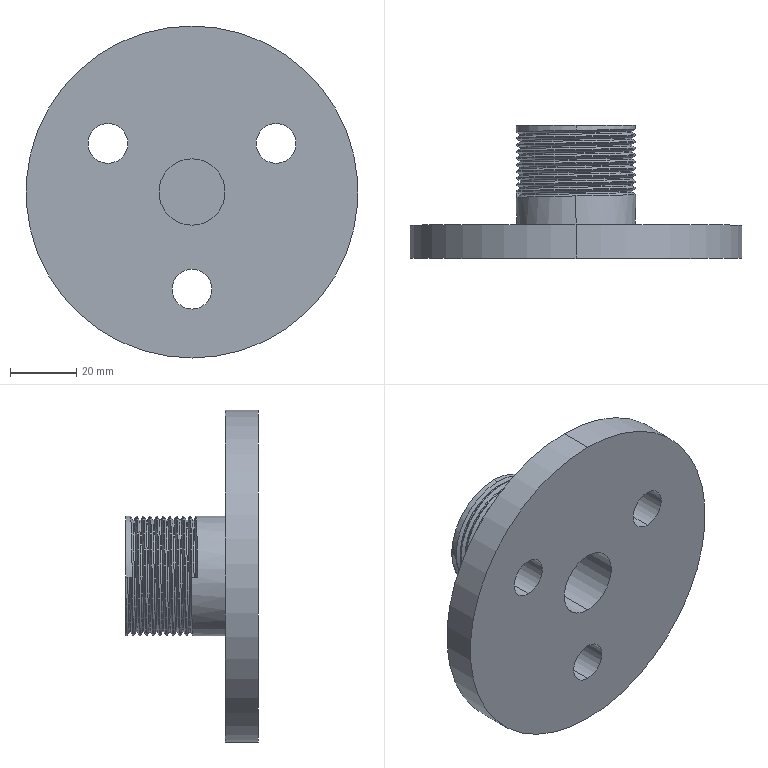Part | SolidWorks | features ICE 3, Extrusion 1, SweepThread 1 | 1 solid | 58 faces | box 100 x 40 x 100 mm | volume 92937 mm3 | cylinder 39 | plane 16 | spline 3 | commonest cylinder face diameters 36 x22 12 x11 20 x4 100 x2